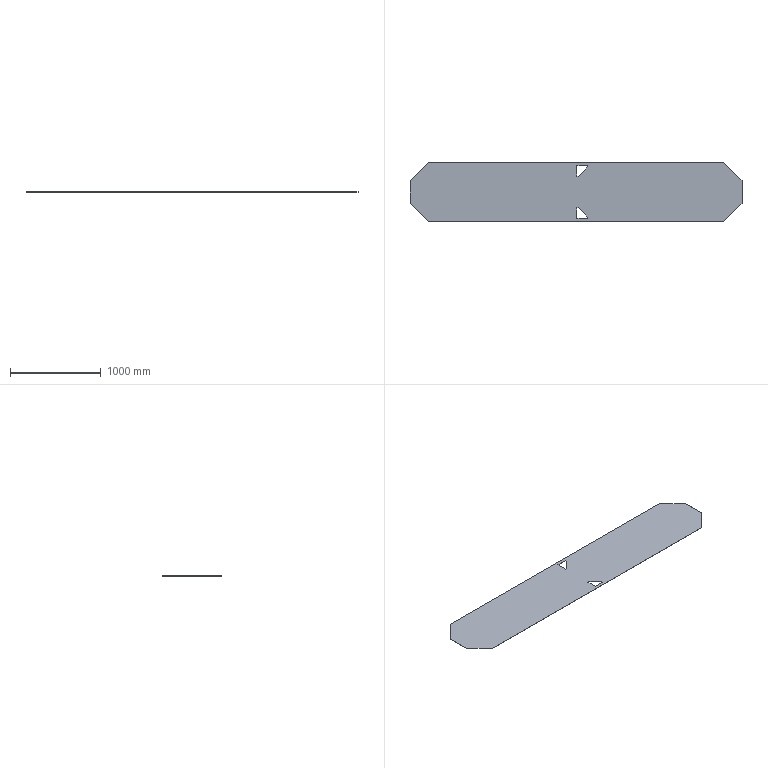Part | STEP file | Bottom weld seal plate2 | 1 solid | 20 faces | box 3650 x 650 x 2 mm | volume 4552100 mm3 | plane 20
STEP:
#1=CARTESIAN_POINT('',(0.,0.,0.));
#2=DIRECTION('',(0.,0.,1.));
#3=DIRECTION('',(1.,0.,0.));
#4=AXIS2_PLACEMENT_3D('',#1,#2,#3);
#5=CARTESIAN_POINT('',(-25.,125.,2.));
#6=VERTEX_POINT('',#5);
#7=CARTESIAN_POINT('',(-25.,-125.,2.));
#8=VERTEX_POINT('',#7);
#9=CARTESIAN_POINT('',(-25.,-125.,2.));
#10=DIRECTION('',(0.,-1.,0.));
#11=VECTOR('',#10,1.);
#12=LINE('',#9,#11);
#13=CARTESIAN_POINT('',(0.,0.,2.));
#14=DIRECTION('',(0.,0.,1.));
#15=DIRECTION('',(1.,0.,0.));
#16=AXIS2_PLACEMENT_3D('',#13,#14,#15);
#17=PLANE('',#16);
#18=CARTESIAN_POINT('',(-25.,-125.));
#19=DIRECTION('',(0.,-1.));
#20=VECTOR('',#19,1.);
#21=LINE('',#18,#20);
#22=(GEOMETRIC_REPRESENTATION_CONTEXT(2)PARAMETRIC_REPRESENTATION_CONTEXT()REPRESENTATION_CONTEXT('',''));
#23=DEFINITIONAL_REPRESENTATION('',(#21),#22);
#24=PCURVE('',#17,#23);
#25=CARTESIAN_POINT('',(-25.,-125.,2.));
#26=DIRECTION('',(1.,0.,0.));
#27=DIRECTION('',(0.,1.,0.));
#28=AXIS2_PLACEMENT_3D('',#25,#26,#27);
#29=PLANE('',#28);
#30=CARTESIAN_POINT('',(0.,0.));
#31=DIRECTION('',(-1.,0.));
#32=VECTOR('',#31,1.);
#33=LINE('',#30,#32);
#34=(GEOMETRIC_REPRESENTATION_CONTEXT(2)PARAMETRIC_REPRESENTATION_CONTEXT()REPRESENTATION_CONTEXT('',''));
#35=DEFINITIONAL_REPRESENTATION('',(#33),#34);
#36=PCURVE('',#29,#35);
#37=SURFACE_CURVE('',#12,(#24,#36),.PCURVE_S1.);
#38=EDGE_CURVE('',#6,#8,#37,.T.);
#39=ORIENTED_EDGE('',*,*,#38,.T.);
#40=CARTESIAN_POINT('',(175.,-325.,2.));
#41=VERTEX_POINT('',#40);
#42=CARTESIAN_POINT('',(-25.,-125.,2.));
#43=DIRECTION('',(0.7071,-0.7071,0.));
#44=VECTOR('',#43,1.);
#45=LINE('',#42,#44);
#46=CARTESIAN_POINT('',(-25.,-125.));
#47=DIRECTION('',(0.7071,-0.7071));
#48=VECTOR('',#47,1.);
#49=LINE('',#46,#48);
#50=(GEOMETRIC_REPRESENTATION_CONTEXT(2)PARAMETRIC_REPRESENTATION_CONTEXT()REPRESENTATION_CONTEXT('',''));
#51=DEFINITIONAL_REPRESENTATION('',(#49),#50);
#52=PCURVE('',#17,#51);
#53=CARTESIAN_POINT('',(-25.,-125.,2.));
#54=DIRECTION('',(0.7071,0.7071,0.));
#55=DIRECTION('',(-0.7071,0.7071,0.));
#56=AXIS2_PLACEMENT_3D('',#53,#54,#55);
#57=PLANE('',#56);
#58=CARTESIAN_POINT('',(0.,0.));
#59=DIRECTION('',(-1.,0.));
#60=VECTOR('',#59,1.);
#61=LINE('',#58,#60);
#62=(GEOMETRIC_REPRESENTATION_CONTEXT(2)PARAMETRIC_REPRESENTATION_CONTEXT()REPRESENTATION_CONTEXT('',''));
#63=DEFINITIONAL_REPRESENTATION('',(#61),#62);
#64=PCURVE('',#57,#63);
#65=SURFACE_CURVE('',#45,(#52,#64),.PCURVE_S1.);
#66=EDGE_CURVE('',#8,#41,#65,.T.);
#67=ORIENTED_EDGE('',*,*,#66,.T.);
#68=CARTESIAN_POINT('',(3425.,-325.,2.));
#69=VERTEX_POINT('',#68);
#70=CARTESIAN_POINT('',(175.,-325.,2.));
#71=DIRECTION('',(1.,0.,0.));
#72=VECTOR('',#71,1.);
#73=LINE('',#70,#72);
#74=CARTESIAN_POINT('',(175.,-325.));
#75=DIRECTION('',(1.,0.));
#76=VECTOR('',#75,1.);
#77=LINE('',#74,#76);
#78=(GEOMETRIC_REPRESENTATION_CONTEXT(2)PARAMETRIC_REPRESENTATION_CONTEXT()REPRESENTATION_CONTEXT('',''));
#79=DEFINITIONAL_REPRESENTATION('',(#77),#78);
#80=PCURVE('',#17,#79);
#81=CARTESIAN_POINT('',(175.,-325.,2.));
#82=DIRECTION('',(0.,1.,0.));
#83=DIRECTION('',(0.,0.,1.));
#84=AXIS2_PLACEMENT_3D('',#81,#82,#83);
#85=PLANE('',#84);
#86=CARTESIAN_POINT('',(0.,0.));
#87=DIRECTION('',(0.,1.));
#88=VECTOR('',#87,1.);
#89=LINE('',#86,#88);
#90=(GEOMETRIC_REPRESENTATION_CONTEXT(2)PARAMETRIC_REPRESENTATION_CONTEXT()REPRESENTATION_CONTEXT('',''));
#91=DEFINITIONAL_REPRESENTATION('',(#89),#90);
#92=PCURVE('',#85,#91);
#93=SURFACE_CURVE('',#73,(#80,#92),.PCURVE_S1.);
#94=EDGE_CURVE('',#41,#69,#93,.T.);
#95=ORIENTED_EDGE('',*,*,#94,.T.);
#96=CARTESIAN_POINT('',(3625.,-125.,2.));
#97=VERTEX_POINT('',#96);
#98=CARTESIAN_POINT('',(3425.,-325.,2.));
#99=DIRECTION('',(0.7071,0.7071,0.));
#100=VECTOR('',#99,1.);
#101=LINE('',#98,#100);
#102=CARTESIAN_POINT('',(3425.,-325.));
#103=DIRECTION('',(0.7071,0.7071));
#104=VECTOR('',#103,1.);
#105=LINE('',#102,#104);
#106=(GEOMETRIC_REPRESENTATION_CONTEXT(2)PARAMETRIC_REPRESENTATION_CONTEXT()REPRESENTATION_CONTEXT('',''));
#107=DEFINITIONAL_REPRESENTATION('',(#105),#106);
#108=PCURVE('',#17,#107);
#109=CARTESIAN_POINT('',(3425.,-325.,2.));
#110=DIRECTION('',(-0.7071,0.7071,0.));
#111=DIRECTION('',(-0.7071,-0.7071,0.));
#112=AXIS2_PLACEMENT_3D('',#109,#110,#111);
#113=PLANE('',#112);
#114=CARTESIAN_POINT('',(0.,0.));
#115=DIRECTION('',(-1.,0.));
#116=VECTOR('',#115,1.);
#117=LINE('',#114,#116);
#118=(GEOMETRIC_REPRESENTATION_CONTEXT(2)PARAMETRIC_REPRESENTATION_CONTEXT()REPRESENTATION_CONTEXT('',''));
#119=DEFINITIONAL_REPRESENTATION('',(#117),#118);
#120=PCURVE('',#113,#119);
#121=SURFACE_CURVE('',#101,(#108,#120),.PCURVE_S1.);
#122=EDGE_CURVE('',#69,#97,#121,.T.);
#123=ORIENTED_EDGE('',*,*,#122,.T.);
#124=CARTESIAN_POINT('',(3625.,125.,2.));
#125=VERTEX_POINT('',#124);
#126=CARTESIAN_POINT('',(3625.,-125.,2.));
#127=DIRECTION('',(0.,1.,0.));
#128=VECTOR('',#127,1.);
#129=LINE('',#126,#128);
#130=CARTESIAN_POINT('',(3625.,-125.));
#131=DIRECTION('',(0.,1.));
#132=VECTOR('',#131,1.);
#133=LINE('',#130,#132);
#134=(GEOMETRIC_REPRESENTATION_CONTEXT(2)PARAMETRIC_REPRESENTATION_CONTEXT()REPRESENTATION_CONTEXT('',''));
#135=DEFINITIONAL_REPRESENTATION('',(#133),#134);
#136=PCURVE('',#17,#135);
#137=CARTESIAN_POINT('',(3625.,-125.,2.));
#138=DIRECTION('',(-1.,0.,0.));
#139=DIRECTION('',(0.,-1.,0.));
#140=AXIS2_PLACEMENT_3D('',#137,#138,#139);
#141=PLANE('',#140);
#142=CARTESIAN_POINT('',(0.,0.));
#143=DIRECTION('',(-1.,0.));
#144=VECTOR('',#143,1.);
#145=LINE('',#142,#144);
#146=(GEOMETRIC_REPRESENTATION_CONTEXT(2)PARAMETRIC_REPRESENTATION_CONTEXT()REPRESENTATION_CONTEXT('',''));
#147=DEFINITIONAL_REPRESENTATION('',(#145),#146);
#148=PCURVE('',#141,#147);
#149=SURFACE_CURVE('',#129,(#136,#148),.PCURVE_S1.);
#150=EDGE_CURVE('',#97,#125,#149,.T.);
#151=ORIENTED_EDGE('',*,*,#150,.T.);
#152=CARTESIAN_POINT('',(3425.,325.,2.));
#153=VERTEX_POINT('',#152);
#154=CARTESIAN_POINT('',(3625.,125.,2.));
#155=DIRECTION('',(-0.7071,0.7071,0.));
#156=VECTOR('',#155,1.);
#157=LINE('',#154,#156);
#158=CARTESIAN_POINT('',(3625.,125.));
#159=DIRECTION('',(-0.7071,0.7071));
#160=VECTOR('',#159,1.);
#161=LINE('',#158,#160);
#162=(GEOMETRIC_REPRESENTATION_CONTEXT(2)PARAMETRIC_REPRESENTATION_CONTEXT()REPRESENTATION_CONTEXT('',''));
#163=DEFINITIONAL_REPRESENTATION('',(#161),#162);
#164=PCURVE('',#17,#163);
#165=CARTESIAN_POINT('',(3625.,125.,2.));
#166=DIRECTION('',(-0.7071,-0.7071,0.));
#167=DIRECTION('',(0.7071,-0.7071,0.));
#168=AXIS2_PLACEMENT_3D('',#165,#166,#167);
#169=PLANE('',#168);
#170=CARTESIAN_POINT('',(0.,0.));
#171=DIRECTION('',(-1.,0.));
#172=VECTOR('',#171,1.);
#173=LINE('',#170,#172);
#174=(GEOMETRIC_REPRESENTATION_CONTEXT(2)PARAMETRIC_REPRESENTATION_CONTEXT()REPRESENTATION_CONTEXT('',''));
#175=DEFINITIONAL_REPRESENTATION('',(#173),#174);
#176=PCURVE('',#169,#175);
#177=SURFACE_CURVE('',#157,(#164,#176),.PCURVE_S1.);
#178=EDGE_CURVE('',#125,#153,#177,.T.);
#179=ORIENTED_EDGE('',*,*,#178,.T.);
#180=CARTESIAN_POINT('',(175.,325.,2.));
#181=VERTEX_POINT('',#180);
#182=CARTESIAN_POINT('',(3425.,325.,2.));
#183=DIRECTION('',(-1.,0.,0.));
#184=VECTOR('',#183,1.);
#185=LINE('',#182,#184);
#186=CARTESIAN_POINT('',(3425.,325.));
#187=DIRECTION('',(-1.,0.));
#188=VECTOR('',#187,1.);
#189=LINE('',#186,#188);
#190=(GEOMETRIC_REPRESENTATION_CONTEXT(2)PARAMETRIC_REPRESENTATION_CONTEXT()REPRESENTATION_CONTEXT('',''));
#191=DEFINITIONAL_REPRESENTATION('',(#189),#190);
#192=PCURVE('',#17,#191);
#193=CARTESIAN_POINT('',(3425.,325.,2.));
#194=DIRECTION('',(0.,-1.,0.));
#195=DIRECTION('',(1.,0.,0.));
#196=AXIS2_PLACEMENT_3D('',#193,#194,#195);
#197=PLANE('',#196);
#198=CARTESIAN_POINT('',(0.,0.));
#199=DIRECTION('',(-1.,0.));
#200=VECTOR('',#199,1.);
#201=LINE('',#198,#200);
#202=(GEOMETRIC_REPRESENTATION_CONTEXT(2)PARAMETRIC_REPRESENTATION_CONTEXT()REPRESENTATION_CONTEXT('',''));
#203=DEFINITIONAL_REPRESENTATION('',(#201),#202);
#204=PCURVE('',#197,#203);
#205=SURFACE_CURVE('',#185,(#192,#204),.PCURVE_S1.);
#206=EDGE_CURVE('',#153,#181,#205,.T.);
#207=ORIENTED_EDGE('',*,*,#206,.T.);
#208=CARTESIAN_POINT('',(175.,325.,2.));
#209=DIRECTION('',(-0.7071,-0.7071,0.));
#210=VECTOR('',#209,1.);
#211=LINE('',#208,#210);
#212=CARTESIAN_POINT('',(175.,325.));
#213=DIRECTION('',(-0.7071,-0.7071));
#214=VECTOR('',#213,1.);
#215=LINE('',#212,#214);
#216=(GEOMETRIC_REPRESENTATION_CONTEXT(2)PARAMETRIC_REPRESENTATION_CONTEXT()REPRESENTATION_CONTEXT('',''));
#217=DEFINITIONAL_REPRESENTATION('',(#215),#216);
#218=PCURVE('',#17,#217);
#219=CARTESIAN_POINT('',(175.,325.,2.));
#220=DIRECTION('',(0.7071,-0.7071,0.));
#221=DIRECTION('',(0.7071,0.7071,0.));
#222=AXIS2_PLACEMENT_3D('',#219,#220,#221);
#223=PLANE('',#222);
#224=CARTESIAN_POINT('',(0.,0.));
#225=DIRECTION('',(-1.,0.));
#226=VECTOR('',#225,1.);
#227=LINE('',#224,#226);
#228=(GEOMETRIC_REPRESENTATION_CONTEXT(2)PARAMETRIC_REPRESENTATION_CONTEXT()REPRESENTATION_CONTEXT('',''));
#229=DEFINITIONAL_REPRESENTATION('',(#227),#228);
#230=PCURVE('',#223,#229);
#231=SURFACE_CURVE('',#211,(#218,#230),.PCURVE_S1.);
#232=EDGE_CURVE('',#181,#6,#231,.T.);
#233=ORIENTED_EDGE('',*,*,#232,.T.);
#234=EDGE_LOOP('',(#39,#67,#95,#123,#151,#179,#207,#233));
#235=FACE_BOUND('',#234,.T.);
#236=CARTESIAN_POINT('',(1810.,175.,2.));
#237=VERTEX_POINT('',#236);
#238=CARTESIAN_POINT('',(1825.,175.,2.));
#239=VERTEX_POINT('',#238);
#240=CARTESIAN_POINT('',(1825.,175.,2.));
#241=DIRECTION('',(1.,0.,0.));
#242=VECTOR('',#241,1.);
#243=LINE('',#240,#242);
#244=CARTESIAN_POINT('',(1825.,175.));
#245=DIRECTION('',(1.,0.));
#246=VECTOR('',#245,1.);
#247=LINE('',#244,#246);
#248=(GEOMETRIC_REPRESENTATION_CONTEXT(2)PARAMETRIC_REPRESENTATION_CONTEXT()REPRESENTATION_CONTEXT('',''));
#249=DEFINITIONAL_REPRESENTATION('',(#247),#248);
#250=PCURVE('',#17,#249);
#251=CARTESIAN_POINT('',(1825.,175.,2.));
#252=DIRECTION('',(0.,1.,0.));
#253=DIRECTION('',(0.,0.,1.));
#254=AXIS2_PLACEMENT_3D('',#251,#252,#253);
#255=PLANE('',#254);
#256=CARTESIAN_POINT('',(0.,0.));
#257=DIRECTION('',(0.,1.));
#258=VECTOR('',#257,1.);
#259=LINE('',#256,#258);
#260=(GEOMETRIC_REPRESENTATION_CONTEXT(2)PARAMETRIC_REPRESENTATION_CONTEXT()REPRESENTATION_CONTEXT('',''));
#261=DEFINITIONAL_REPRESENTATION('',(#259),#260);
#262=PCURVE('',#255,#261);
#263=SURFACE_CURVE('',#243,(#250,#262),.PCURVE_S1.);
#264=EDGE_CURVE('',#237,#239,#263,.T.);
#265=ORIENTED_EDGE('',*,*,#264,.F.);
#266=CARTESIAN_POINT('',(1810.,290.,2.));
#267=VERTEX_POINT('',#266);
#268=CARTESIAN_POINT('',(1810.,175.,2.));
#269=DIRECTION('',(0.,-1.,0.));
#270=VECTOR('',#269,1.);
#271=LINE('',#268,#270);
#272=CARTESIAN_POINT('',(1810.,175.));
#273=DIRECTION('',(0.,-1.));
#274=VECTOR('',#273,1.);
#275=LINE('',#272,#274);
#276=(GEOMETRIC_REPRESENTATION_CONTEXT(2)PARAMETRIC_REPRESENTATION_CONTEXT()REPRESENTATION_CONTEXT('',''));
#277=DEFINITIONAL_REPRESENTATION('',(#275),#276);
#278=PCURVE('',#17,#277);
#279=CARTESIAN_POINT('',(1810.,175.,2.));
#280=DIRECTION('',(1.,0.,0.));
#281=DIRECTION('',(0.,0.,-1.));
#282=AXIS2_PLACEMENT_3D('',#279,#280,#281);
#283=PLANE('',#282);
#284=CARTESIAN_POINT('',(0.,0.));
#285=DIRECTION('',(0.,-1.));
#286=VECTOR('',#285,1.);
#287=LINE('',#284,#286);
#288=(GEOMETRIC_REPRESENTATION_CONTEXT(2)PARAMETRIC_REPRESENTATION_CONTEXT()REPRESENTATION_CONTEXT('',''));
#289=DEFINITIONAL_REPRESENTATION('',(#287),#288);
#290=PCURVE('',#283,#289);
#291=SURFACE_CURVE('',#271,(#278,#290),.PCURVE_S1.);
#292=EDGE_CURVE('',#267,#237,#291,.T.);
#293=ORIENTED_EDGE('',*,*,#292,.F.);
#294=CARTESIAN_POINT('',(1925.,290.,2.));
#295=VERTEX_POINT('',#294);
#296=CARTESIAN_POINT('',(1810.,290.,2.));
#297=DIRECTION('',(-1.,0.,0.));
#298=VECTOR('',#297,1.);
#299=LINE('',#296,#298);
#300=CARTESIAN_POINT('',(1810.,290.));
#301=DIRECTION('',(-1.,0.));
#302=VECTOR('',#301,1.);
#303=LINE('',#300,#302);
#304=(GEOMETRIC_REPRESENTATION_CONTEXT(2)PARAMETRIC_REPRESENTATION_CONTEXT()REPRESENTATION_CONTEXT('',''));
#305=DEFINITIONAL_REPRESENTATION('',(#303),#304);
#306=PCURVE('',#17,#305);
#307=CARTESIAN_POINT('',(1810.,290.,2.));
#308=DIRECTION('',(0.,-1.,0.));
#309=DIRECTION('',(0.,0.,-1.));
#310=AXIS2_PLACEMENT_3D('',#307,#308,#309);
#311=PLANE('',#310);
#312=CARTESIAN_POINT('',(0.,0.));
#313=DIRECTION('',(0.,-1.));
#314=VECTOR('',#313,1.);
#315=LINE('',#312,#314);
#316=(GEOMETRIC_REPRESENTATION_CONTEXT(2)PARAMETRIC_REPRESENTATION_CONTEXT()REPRESENTATION_CONTEXT('',''));
#317=DEFINITIONAL_REPRESENTATION('',(#315),#316);
#318=PCURVE('',#311,#317);
#319=SURFACE_CURVE('',#299,(#306,#318),.PCURVE_S1.);
#320=EDGE_CURVE('',#295,#267,#319,.T.);
#321=ORIENTED_EDGE('',*,*,#320,.F.);
#322=CARTESIAN_POINT('',(1925.,275.,2.));
#323=VERTEX_POINT('',#322);
#324=CARTESIAN_POINT('',(1925.,290.,2.));
#325=DIRECTION('',(0.,1.,0.));
#326=VECTOR('',#325,1.);
#327=LINE('',#324,#326);
#328=CARTESIAN_POINT('',(1925.,290.));
#329=DIRECTION('',(0.,1.));
#330=VECTOR('',#329,1.);
#331=LINE('',#328,#330);
#332=(GEOMETRIC_REPRESENTATION_CONTEXT(2)PARAMETRIC_REPRESENTATION_CONTEXT()REPRESENTATION_CONTEXT('',''));
#333=DEFINITIONAL_REPRESENTATION('',(#331),#332);
#334=PCURVE('',#17,#333);
#335=CARTESIAN_POINT('',(1925.,290.,2.));
#336=DIRECTION('',(-1.,0.,0.));
#337=DIRECTION('',(0.,0.,1.));
#338=AXIS2_PLACEMENT_3D('',#335,#336,#337);
#339=PLANE('',#338);
#340=CARTESIAN_POINT('',(0.,0.));
#341=DIRECTION('',(0.,1.));
#342=VECTOR('',#341,1.);
#343=LINE('',#340,#342);
#344=(GEOMETRIC_REPRESENTATION_CONTEXT(2)PARAMETRIC_REPRESENTATION_CONTEXT()REPRESENTATION_CONTEXT('',''));
#345=DEFINITIONAL_REPRESENTATION('',(#343),#344);
#346=PCURVE('',#339,#345);
#347=SURFACE_CURVE('',#327,(#334,#346),.PCURVE_S1.);
#348=EDGE_CURVE('',#323,#295,#347,.T.);
#349=ORIENTED_EDGE('',*,*,#348,.F.);
#350=CARTESIAN_POINT('',(1925.,275.,2.));
#351=DIRECTION('',(0.7071,0.7071,0.));
#352=VECTOR('',#351,1.);
#353=LINE('',#350,#352);
#354=CARTESIAN_POINT('',(1925.,275.));
#355=DIRECTION('',(0.7071,0.7071));
#356=VECTOR('',#355,1.);
#357=LINE('',#354,#356);
#358=(GEOMETRIC_REPRESENTATION_CONTEXT(2)PARAMETRIC_REPRESENTATION_CONTEXT()REPRESENTATION_CONTEXT('',''));
#359=DEFINITIONAL_REPRESENTATION('',(#357),#358);
#360=PCURVE('',#17,#359);
#361=CARTESIAN_POINT('',(1925.,275.,2.));
#362=DIRECTION('',(-0.7071,0.7071,0.));
#363=DIRECTION('',(-0.7071,-0.7071,0.));
#364=AXIS2_PLACEMENT_3D('',#361,#362,#363);
#365=PLANE('',#364);
#366=CARTESIAN_POINT('',(0.,0.));
#367=DIRECTION('',(-1.,0.));
#368=VECTOR('',#367,1.);
#369=LINE('',#366,#368);
#370=(GEOMETRIC_REPRESENTATION_CONTEXT(2)PARAMETRIC_REPRESENTATION_CONTEXT()REPRESENTATION_CONTEXT('',''));
#371=DEFINITIONAL_REPRESENTATION('',(#369),#370);
#372=PCURVE('',#365,#371);
#373=SURFACE_CURVE('',#353,(#360,#372),.PCURVE_S1.);
#374=EDGE_CURVE('',#239,#323,#373,.T.);
#375=ORIENTED_EDGE('',*,*,#374,.F.);
#376=EDGE_LOOP('',(#265,#293,#321,#349,#375));
#377=FACE_BOUND('',#376,.T.);
#378=CARTESIAN_POINT('',(1925.,-290.,2.));
#379=VERTEX_POINT('',#378);
#380=CARTESIAN_POINT('',(1925.,-275.,2.));
#381=VERTEX_POINT('',#380);
#382=CARTESIAN_POINT('',(1925.,-290.,2.));
#383=DIRECTION('',(0.,1.,0.));
#384=VECTOR('',#383,1.);
#385=LINE('',#382,#384);
#386=CARTESIAN_POINT('',(1925.,-290.));
#387=DIRECTION('',(0.,1.));
#388=VECTOR('',#387,1.);
#389=LINE('',#386,#388);
#390=(GEOMETRIC_REPRESENTATION_CONTEXT(2)PARAMETRIC_REPRESENTATION_CONTEXT()REPRESENTATION_CONTEXT('',''));
#391=DEFINITIONAL_REPRESENTATION('',(#389),#390);
#392=PCURVE('',#17,#391);
#393=CARTESIAN_POINT('',(1925.,-290.,2.));
#394=DIRECTION('',(-1.,0.,0.));
#395=DIRECTION('',(0.,0.,1.));
#396=AXIS2_PLACEMENT_3D('',#393,#394,#395);
#397=PLANE('',#396);
#398=CARTESIAN_POINT('',(0.,0.));
#399=DIRECTION('',(0.,1.));
#400=VECTOR('',#399,1.);
#401=LINE('',#398,#400);
#402=(GEOMETRIC_REPRESENTATION_CONTEXT(2)PARAMETRIC_REPRESENTATION_CONTEXT()REPRESENTATION_CONTEXT('',''));
#403=DEFINITIONAL_REPRESENTATION('',(#401),#402);
#404=PCURVE('',#397,#403);
#405=SURFACE_CURVE('',#385,(#392,#404),.PCURVE_S1.);
#406=EDGE_CURVE('',#379,#381,#405,.T.);
#407=ORIENTED_EDGE('',*,*,#406,.F.);
#408=CARTESIAN_POINT('',(1810.,-290.,2.));
#409=VERTEX_POINT('',#408);
#410=CARTESIAN_POINT('',(1810.,-290.,2.));
#411=DIRECTION('',(1.,0.,0.));
#412=VECTOR('',#411,1.);
#413=LINE('',#410,#412);
#414=CARTESIAN_POINT('',(1810.,-290.));
#415=DIRECTION('',(1.,0.));
#416=VECTOR('',#415,1.);
#417=LINE('',#414,#416);
#418=(GEOMETRIC_REPRESENTATION_CONTEXT(2)PARAMETRIC_REPRESENTATION_CONTEXT()REPRESENTATION_CONTEXT('',''));
#419=DEFINITIONAL_REPRESENTATION('',(#417),#418);
#420=PCURVE('',#17,#419);
#421=CARTESIAN_POINT('',(1810.,-290.,2.));
#422=DIRECTION('',(0.,1.,0.));
#423=DIRECTION('',(0.,0.,1.));
#424=AXIS2_PLACEMENT_3D('',#421,#422,#423);
#425=PLANE('',#424);
#426=CARTESIAN_POINT('',(0.,0.));
#427=DIRECTION('',(0.,1.));
#428=VECTOR('',#427,1.);
#429=LINE('',#426,#428);
#430=(GEOMETRIC_REPRESENTATION_CONTEXT(2)PARAMETRIC_REPRESENTATION_CONTEXT()REPRESENTATION_CONTEXT('',''));
#431=DEFINITIONAL_REPRESENTATION('',(#429),#430);
#432=PCURVE('',#425,#431);
#433=SURFACE_CURVE('',#413,(#420,#432),.PCURVE_S1.);
#434=EDGE_CURVE('',#409,#379,#433,.T.);
#435=ORIENTED_EDGE('',*,*,#434,.F.);
#436=CARTESIAN_POINT('',(1810.,-175.,2.));
#437=VERTEX_POINT('',#436);
#438=CARTESIAN_POINT('',(1810.,-290.,2.));
#439=DIRECTION('',(0.,-1.,0.));
#440=VECTOR('',#439,1.);
#441=LINE('',#438,#440);
#442=CARTESIAN_POINT('',(1810.,-290.));
#443=DIRECTION('',(0.,-1.));
#444=VECTOR('',#443,1.);
#445=LINE('',#442,#444);
#446=(GEOMETRIC_REPRESENTATION_CONTEXT(2)PARAMETRIC_REPRESENTATION_CONTEXT()REPRESENTATION_CONTEXT('',''));
#447=DEFINITIONAL_REPRESENTATION('',(#445),#446);
#448=PCURVE('',#17,#447);
#449=CARTESIAN_POINT('',(1810.,-290.,2.));
#450=DIRECTION('',(1.,0.,0.));
#451=DIRECTION('',(0.,0.,-1.));
#452=AXIS2_PLACEMENT_3D('',#449,#450,#451);
#453=PLANE('',#452);
#454=CARTESIAN_POINT('',(0.,0.));
#455=DIRECTION('',(0.,-1.));
#456=VECTOR('',#455,1.);
#457=LINE('',#454,#456);
#458=(GEOMETRIC_REPRESENTATION_CONTEXT(2)PARAMETRIC_REPRESENTATION_CONTEXT()REPRESENTATION_CONTEXT('',''));
#459=DEFINITIONAL_REPRESENTATION('',(#457),#458);
#460=PCURVE('',#453,#459);
#461=SURFACE_CURVE('',#441,(#448,#460),.PCURVE_S1.);
#462=EDGE_CURVE('',#437,#409,#461,.T.);
#463=ORIENTED_EDGE('',*,*,#462,.F.);
#464=CARTESIAN_POINT('',(1825.,-175.,2.));
#465=VERTEX_POINT('',#464);
#466=CARTESIAN_POINT('',(1825.,-175.,2.));
#467=DIRECTION('',(-1.,0.,0.));
#468=VECTOR('',#467,1.);
#469=LINE('',#466,#468);
#470=CARTESIAN_POINT('',(1825.,-175.));
#471=DIRECTION('',(-1.,0.));
#472=VECTOR('',#471,1.);
#473=LINE('',#470,#472);
#474=(GEOMETRIC_REPRESENTATION_CONTEXT(2)PARAMETRIC_REPRESENTATION_CONTEXT()REPRESENTATION_CONTEXT('',''));
#475=DEFINITIONAL_REPRESENTATION('',(#473),#474);
#476=PCURVE('',#17,#475);
#477=CARTESIAN_POINT('',(1825.,-175.,2.));
#478=DIRECTION('',(0.,-1.,0.));
#479=DIRECTION('',(0.,0.,-1.));
#480=AXIS2_PLACEMENT_3D('',#477,#478,#479);
#481=PLANE('',#480);
#482=CARTESIAN_POINT('',(0.,0.));
#483=DIRECTION('',(0.,-1.));
#484=VECTOR('',#483,1.);
#485=LINE('',#482,#484);
#486=(GEOMETRIC_REPRESENTATION_CONTEXT(2)PARAMETRIC_REPRESENTATION_CONTEXT()REPRESENTATION_CONTEXT('',''));
#487=DEFINITIONAL_REPRESENTATION('',(#485),#486);
#488=PCURVE('',#481,#487);
#489=SURFACE_CURVE('',#469,(#476,#488),.PCURVE_S1.);
#490=EDGE_CURVE('',#465,#437,#489,.T.);
#491=ORIENTED_EDGE('',*,*,#490,.F.);
#492=CARTESIAN_POINT('',(1925.,-275.,2.));
#493=DIRECTION('',(-0.7071,0.7071,0.));
#494=VECTOR('',#493,1.);
#495=LINE('',#492,#494);
#496=CARTESIAN_POINT('',(1925.,-275.));
#497=DIRECTION('',(-0.7071,0.7071));
#498=VECTOR('',#497,1.);
#499=LINE('',#496,#498);
#500=(GEOMETRIC_REPRESENTATION_CONTEXT(2)PARAMETRIC_REPRESENTATION_CONTEXT()REPRESENTATION_CONTEXT('',''));
#501=DEFINITIONAL_REPRESENTATION('',(#499),#500);
#502=PCURVE('',#17,#501);
#503=CARTESIAN_POINT('',(1925.,-275.,2.));
#504=DIRECTION('',(-0.7071,-0.7071,0.));
#505=DIRECTION('',(0.7071,-0.7071,0.));
#506=AXIS2_PLACEMENT_3D('',#503,#504,#505);
#507=PLANE('',#506);
#508=CARTESIAN_POINT('',(0.,0.));
#509=DIRECTION('',(-1.,0.));
#510=VECTOR('',#509,1.);
#511=LINE('',#508,#510);
#512=(GEOMETRIC_REPRESENTATION_CONTEXT(2)PARAMETRIC_REPRESENTATION_CONTEXT()REPRESENTATION_CONTEXT('',''));
#513=DEFINITIONAL_REPRESENTATION('',(#511),#512);
#514=PCURVE('',#507,#513);
#515=SURFACE_CURVE('',#495,(#502,#514),.PCURVE_S1.);
#516=EDGE_CURVE('',#381,#465,#515,.T.);
#517=ORIENTED_EDGE('',*,*,#516,.F.);
#518=EDGE_LOOP('',(#407,#435,#463,#491,#517));
#519=FACE_BOUND('',#518,.T.);
#520=ADVANCED_FACE('',(#235,#377,#519),#17,.T.);
#521=CARTESIAN_POINT('',(1810.,290.,0.));
#522=VERTEX_POINT('',#521);
#523=CARTESIAN_POINT('',(1810.,175.,0.));
#524=VERTEX_POINT('',#523);
#525=CARTESIAN_POINT('',(1810.,175.,0.));
#526=DIRECTION('',(0.,-1.,0.));
#527=VECTOR('',#526,1.);
#528=LINE('',#525,#527);
#529=CARTESIAN_POINT('',(0.,0.,0.));
#530=DIRECTION('',(0.,0.,1.));
#531=DIRECTION('',(1.,0.,0.));
#532=AXIS2_PLACEMENT_3D('',#529,#530,#531);
#533=PLANE('',#532);
#534=CARTESIAN_POINT('',(1810.,175.));
#535=DIRECTION('',(0.,-1.));
#536=VECTOR('',#535,1.);
#537=LINE('',#534,#536);
#538=(GEOMETRIC_REPRESENTATION_CONTEXT(2)PARAMETRIC_REPRESENTATION_CONTEXT()REPRESENTATION_CONTEXT('',''));
#539=DEFINITIONAL_REPRESENTATION('',(#537),#538);
#540=PCURVE('',#533,#539);
#541=CARTESIAN_POINT('',(2.,0.));
#542=DIRECTION('',(0.,-1.));
#543=VECTOR('',#542,1.);
#544=LINE('',#541,#543);
#545=(GEOMETRIC_REPRESENTATION_CONTEXT(2)PARAMETRIC_REPRESENTATION_CONTEXT()REPRESENTATION_CONTEXT('',''));
#546=DEFINITIONAL_REPRESENTATION('',(#544),#545);
#547=PCURVE('',#283,#546);
#548=SURFACE_CURVE('',#528,(#540,#547),.PCURVE_S1.);
#549=EDGE_CURVE('',#522,#524,#548,.T.);
#550=ORIENTED_EDGE('',*,*,#549,.T.);
#551=CARTESIAN_POINT('',(1825.,175.,0.));
#552=VERTEX_POINT('',#551);
#553=CARTESIAN_POINT('',(1825.,175.,0.));
#554=DIRECTION('',(1.,0.,0.));
#555=VECTOR('',#554,1.);
#556=LINE('',#553,#555);
#557=CARTESIAN_POINT('',(1825.,175.));
#558=DIRECTION('',(1.,0.));
#559=VECTOR('',#558,1.);
#560=LINE('',#557,#559);
#561=(GEOMETRIC_REPRESENTATION_CONTEXT(2)PARAMETRIC_REPRESENTATION_CONTEXT()REPRESENTATION_CONTEXT('',''));
#562=DEFINITIONAL_REPRESENTATION('',(#560),#561);
#563=PCURVE('',#533,#562);
#564=CARTESIAN_POINT('',(-2.,0.));
#565=DIRECTION('',(0.,1.));
#566=VECTOR('',#565,1.);
#567=LINE('',#564,#566);
#568=(GEOMETRIC_REPRESENTATION_CONTEXT(2)PARAMETRIC_REPRESENTATION_CONTEXT()REPRESENTATION_CONTEXT('',''));
#569=DEFINITIONAL_REPRESENTATION('',(#567),#568);
#570=PCURVE('',#255,#569);
#571=SURFACE_CURVE('',#556,(#563,#570),.PCURVE_S1.);
#572=EDGE_CURVE('',#524,#552,#571,.T.);
#573=ORIENTED_EDGE('',*,*,#572,.T.);
#574=CARTESIAN_POINT('',(1925.,275.,0.));
#575=VERTEX_POINT('',#574);
#576=CARTESIAN_POINT('',(1925.,275.,0.));
#577=DIRECTION('',(0.7071,0.7071,0.));
#578=VECTOR('',#577,1.);
#579=LINE('',#576,#578);
#580=CARTESIAN_POINT('',(1925.,275.));
#581=DIRECTION('',(0.7071,0.7071));
#582=VECTOR('',#581,1.);
#583=LINE('',#580,#582);
#584=(GEOMETRIC_REPRESENTATION_CONTEXT(2)PARAMETRIC_REPRESENTATION_CONTEXT()REPRESENTATION_CONTEXT('',''));
#585=DEFINITIONAL_REPRESENTATION('',(#583),#584);
#586=PCURVE('',#533,#585);
#587=CARTESIAN_POINT('',(0.,-2.));
#588=DIRECTION('',(-1.,0.));
#589=VECTOR('',#588,1.);
#590=LINE('',#587,#589);
#591=(GEOMETRIC_REPRESENTATION_CONTEXT(2)PARAMETRIC_REPRESENTATION_CONTEXT()REPRESENTATION_CONTEXT('',''));
#592=DEFINITIONAL_REPRESENTATION('',(#590),#591);
#593=PCURVE('',#365,#592);
#594=SURFACE_CURVE('',#579,(#586,#593),.PCURVE_S1.);
#595=EDGE_CURVE('',#552,#575,#594,.T.);
#596=ORIENTED_EDGE('',*,*,#595,.T.);
#597=CARTESIAN_POINT('',(1925.,290.,0.));
#598=VERTEX_POINT('',#597);
#599=CARTESIAN_POINT('',(1925.,290.,0.));
#600=DIRECTION('',(0.,1.,0.));
#601=VECTOR('',#600,1.);
#602=LINE('',#599,#601);
#603=CARTESIAN_POINT('',(1925.,290.));
#604=DIRECTION('',(0.,1.));
#605=VECTOR('',#604,1.);
#606=LINE('',#603,#605);
#607=(GEOMETRIC_REPRESENTATION_CONTEXT(2)PARAMETRIC_REPRESENTATION_CONTEXT()REPRESENTATION_CONTEXT('',''));
#608=DEFINITIONAL_REPRESENTATION('',(#606),#607);
#609=PCURVE('',#533,#608);
#610=CARTESIAN_POINT('',(-2.,0.));
#611=DIRECTION('',(0.,1.));
#612=VECTOR('',#611,1.);
#613=LINE('',#610,#612);
#614=(GEOMETRIC_REPRESENTATION_CONTEXT(2)PARAMETRIC_REPRESENTATION_CONTEXT()REPRESENTATION_CONTEXT('',''));
#615=DEFINITIONAL_REPRESENTATION('',(#613),#614);
#616=PCURVE('',#339,#615);
#617=SURFACE_CURVE('',#602,(#609,#616),.PCURVE_S1.);
#618=EDGE_CURVE('',#575,#598,#617,.T.);
#619=ORIENTED_EDGE('',*,*,#618,.T.);
#620=CARTESIAN_POINT('',(1810.,290.,0.));
#621=DIRECTION('',(-1.,0.,0.));
#622=VECTOR('',#621,1.);
#623=LINE('',#620,#622);
#624=CARTESIAN_POINT('',(1810.,290.));
#625=DIRECTION('',(-1.,0.));
#626=VECTOR('',#625,1.);
#627=LINE('',#624,#626);
#628=(GEOMETRIC_REPRESENTATION_CONTEXT(2)PARAMETRIC_REPRESENTATION_CONTEXT()REPRESENTATION_CONTEXT('',''));
#629=DEFINITIONAL_REPRESENTATION('',(#627),#628);
#630=PCURVE('',#533,#629);
#631=CARTESIAN_POINT('',(2.,0.));
#632=DIRECTION('',(0.,-1.));
#633=VECTOR('',#632,1.);
#634=LINE('',#631,#633);
#635=(GEOMETRIC_REPRESENTATION_CONTEXT(2)PARAMETRIC_REPRESENTATION_CONTEXT()REPRESENTATION_CONTEXT('',''));
#636=DEFINITIONAL_REPRESENTATION('',(#634),#635);
#637=PCURVE('',#311,#636);
#638=SURFACE_CURVE('',#623,(#630,#637),.PCURVE_S1.);
#639=EDGE_CURVE('',#598,#522,#638,.T.);
#640=ORIENTED_EDGE('',*,*,#639,.T.);
#641=EDGE_LOOP('',(#550,#573,#596,#619,#640));
#642=FACE_BOUND('',#641,.T.);
#643=CARTESIAN_POINT('',(-25.,125.,0.));
#644=VERTEX_POINT('',#643);
#645=CARTESIAN_POINT('',(-25.,-125.,0.));
#646=VERTEX_POINT('',#645);
#647=CARTESIAN_POINT('',(-25.,-125.,0.));
#648=DIRECTION('',(0.,-1.,0.));
#649=VECTOR('',#648,1.);
#650=LINE('',#647,#649);
#651=CARTESIAN_POINT('',(-25.,-125.));
#652=DIRECTION('',(0.,-1.));
#653=VECTOR('',#652,1.);
#654=LINE('',#651,#653);
#655=(GEOMETRIC_REPRESENTATION_CONTEXT(2)PARAMETRIC_REPRESENTATION_CONTEXT()REPRESENTATION_CONTEXT('',''));
#656=DEFINITIONAL_REPRESENTATION('',(#654),#655);
#657=PCURVE('',#533,#656);
#658=CARTESIAN_POINT('',(0.,-2.));
#659=DIRECTION('',(-1.,0.));
#660=VECTOR('',#659,1.);
#661=LINE('',#658,#660);
#662=(GEOMETRIC_REPRESENTATION_CONTEXT(2)PARAMETRIC_REPRESENTATION_CONTEXT()REPRESENTATION_CONTEXT('',''));
#663=DEFINITIONAL_REPRESENTATION('',(#661),#662);
#664=PCURVE('',#29,#663);
#665=SURFACE_CURVE('',#650,(#657,#664),.PCURVE_S1.);
#666=EDGE_CURVE('',#644,#646,#665,.T.);
#667=ORIENTED_EDGE('',*,*,#666,.F.);
#668=CARTESIAN_POINT('',(175.,325.,0.));
#669=VERTEX_POINT('',#668);
#670=CARTESIAN_POINT('',(175.,325.,0.));
#671=DIRECTION('',(-0.7071,-0.7071,0.));
#672=VECTOR('',#671,1.);
#673=LINE('',#670,#672);
#674=CARTESIAN_POINT('',(175.,325.));
#675=DIRECTION('',(-0.7071,-0.7071));
#676=VECTOR('',#675,1.);
#677=LINE('',#674,#676);
#678=(GEOMETRIC_REPRESENTATION_CONTEXT(2)PARAMETRIC_REPRESENTATION_CONTEXT()REPRESENTATION_CONTEXT('',''));
#679=DEFINITIONAL_REPRESENTATION('',(#677),#678);
#680=PCURVE('',#533,#679);
#681=CARTESIAN_POINT('',(0.,-2.));
#682=DIRECTION('',(-1.,0.));
#683=VECTOR('',#682,1.);
#684=LINE('',#681,#683);
#685=(GEOMETRIC_REPRESENTATION_CONTEXT(2)PARAMETRIC_REPRESENTATION_CONTEXT()REPRESENTATION_CONTEXT('',''));
#686=DEFINITIONAL_REPRESENTATION('',(#684),#685);
#687=PCURVE('',#223,#686);
#688=SURFACE_CURVE('',#673,(#680,#687),.PCURVE_S1.);
#689=EDGE_CURVE('',#669,#644,#688,.T.);
#690=ORIENTED_EDGE('',*,*,#689,.F.);
#691=CARTESIAN_POINT('',(3425.,325.,0.));
#692=VERTEX_POINT('',#691);
#693=CARTESIAN_POINT('',(3425.,325.,0.));
#694=DIRECTION('',(-1.,0.,0.));
#695=VECTOR('',#694,1.);
#696=LINE('',#693,#695);
#697=CARTESIAN_POINT('',(3425.,325.));
#698=DIRECTION('',(-1.,0.));
#699=VECTOR('',#698,1.);
#700=LINE('',#697,#699);
#701=(GEOMETRIC_REPRESENTATION_CONTEXT(2)PARAMETRIC_REPRESENTATION_CONTEXT()REPRESENTATION_CONTEXT('',''));
#702=DEFINITIONAL_REPRESENTATION('',(#700),#701);
#703=PCURVE('',#533,#702);
#704=CARTESIAN_POINT('',(0.,-2.));
#705=DIRECTION('',(-1.,0.));
#706=VECTOR('',#705,1.);
#707=LINE('',#704,#706);
#708=(GEOMETRIC_REPRESENTATION_CONTEXT(2)PARAMETRIC_REPRESENTATION_CONTEXT()REPRESENTATION_CONTEXT('',''));
#709=DEFINITIONAL_REPRESENTATION('',(#707),#708);
#710=PCURVE('',#197,#709);
#711=SURFACE_CURVE('',#696,(#703,#710),.PCURVE_S1.);
#712=EDGE_CURVE('',#692,#669,#711,.T.);
#713=ORIENTED_EDGE('',*,*,#712,.F.);
#714=CARTESIAN_POINT('',(3625.,125.,0.));
#715=VERTEX_POINT('',#714);
#716=CARTESIAN_POINT('',(3625.,125.,0.));
#717=DIRECTION('',(-0.7071,0.7071,0.));
#718=VECTOR('',#717,1.);
#719=LINE('',#716,#718);
#720=CARTESIAN_POINT('',(3625.,125.));
#721=DIRECTION('',(-0.7071,0.7071));
#722=VECTOR('',#721,1.);
#723=LINE('',#720,#722);
#724=(GEOMETRIC_REPRESENTATION_CONTEXT(2)PARAMETRIC_REPRESENTATION_CONTEXT()REPRESENTATION_CONTEXT('',''));
#725=DEFINITIONAL_REPRESENTATION('',(#723),#724);
#726=PCURVE('',#533,#725);
#727=CARTESIAN_POINT('',(0.,-2.));
#728=DIRECTION('',(-1.,0.));
#729=VECTOR('',#728,1.);
#730=LINE('',#727,#729);
#731=(GEOMETRIC_REPRESENTATION_CONTEXT(2)PARAMETRIC_REPRESENTATION_CONTEXT()REPRESENTATION_CONTEXT('',''));
#732=DEFINITIONAL_REPRESENTATION('',(#730),#731);
#733=PCURVE('',#169,#732);
#734=SURFACE_CURVE('',#719,(#726,#733),.PCURVE_S1.);
#735=EDGE_CURVE('',#715,#692,#734,.T.);
#736=ORIENTED_EDGE('',*,*,#735,.F.);
#737=CARTESIAN_POINT('',(3625.,-125.,0.));
#738=VERTEX_POINT('',#737);
#739=CARTESIAN_POINT('',(3625.,-125.,0.));
#740=DIRECTION('',(0.,1.,0.));
#741=VECTOR('',#740,1.);
#742=LINE('',#739,#741);
#743=CARTESIAN_POINT('',(3625.,-125.));
#744=DIRECTION('',(0.,1.));
#745=VECTOR('',#744,1.);
#746=LINE('',#743,#745);
#747=(GEOMETRIC_REPRESENTATION_CONTEXT(2)PARAMETRIC_REPRESENTATION_CONTEXT()REPRESENTATION_CONTEXT('',''));
#748=DEFINITIONAL_REPRESENTATION('',(#746),#747);
#749=PCURVE('',#533,#748);
#750=CARTESIAN_POINT('',(0.,-2.));
#751=DIRECTION('',(-1.,0.));
#752=VECTOR('',#751,1.);
#753=LINE('',#750,#752);
#754=(GEOMETRIC_REPRESENTATION_CONTEXT(2)PARAMETRIC_REPRESENTATION_CONTEXT()REPRESENTATION_CONTEXT('',''));
#755=DEFINITIONAL_REPRESENTATION('',(#753),#754);
#756=PCURVE('',#141,#755);
#757=SURFACE_CURVE('',#742,(#749,#756),.PCURVE_S1.);
#758=EDGE_CURVE('',#738,#715,#757,.T.);
#759=ORIENTED_EDGE('',*,*,#758,.F.);
#760=CARTESIAN_POINT('',(3425.,-325.,0.));
#761=VERTEX_POINT('',#760);
#762=CARTESIAN_POINT('',(3425.,-325.,0.));
#763=DIRECTION('',(0.7071,0.7071,0.));
#764=VECTOR('',#763,1.);
#765=LINE('',#762,#764);
#766=CARTESIAN_POINT('',(3425.,-325.));
#767=DIRECTION('',(0.7071,0.7071));
#768=VECTOR('',#767,1.);
#769=LINE('',#766,#768);
#770=(GEOMETRIC_REPRESENTATION_CONTEXT(2)PARAMETRIC_REPRESENTATION_CONTEXT()REPRESENTATION_CONTEXT('',''));
#771=DEFINITIONAL_REPRESENTATION('',(#769),#770);
#772=PCURVE('',#533,#771);
#773=CARTESIAN_POINT('',(0.,-2.));
#774=DIRECTION('',(-1.,0.));
#775=VECTOR('',#774,1.);
#776=LINE('',#773,#775);
#777=(GEOMETRIC_REPRESENTATION_CONTEXT(2)PARAMETRIC_REPRESENTATION_CONTEXT()REPRESENTATION_CONTEXT('',''));
#778=DEFINITIONAL_REPRESENTATION('',(#776),#777);
#779=PCURVE('',#113,#778);
#780=SURFACE_CURVE('',#765,(#772,#779),.PCURVE_S1.);
#781=EDGE_CURVE('',#761,#738,#780,.T.);
#782=ORIENTED_EDGE('',*,*,#781,.F.);
#783=CARTESIAN_POINT('',(175.,-325.,0.));
#784=VERTEX_POINT('',#783);
#785=CARTESIAN_POINT('',(175.,-325.,0.));
#786=DIRECTION('',(1.,0.,0.));
#787=VECTOR('',#786,1.);
#788=LINE('',#785,#787);
#789=CARTESIAN_POINT('',(175.,-325.));
#790=DIRECTION('',(1.,0.));
#791=VECTOR('',#790,1.);
#792=LINE('',#789,#791);
#793=(GEOMETRIC_REPRESENTATION_CONTEXT(2)PARAMETRIC_REPRESENTATION_CONTEXT()REPRESENTATION_CONTEXT('',''));
#794=DEFINITIONAL_REPRESENTATION('',(#792),#793);
#795=PCURVE('',#533,#794);
#796=CARTESIAN_POINT('',(-2.,0.));
#797=DIRECTION('',(0.,1.));
#798=VECTOR('',#797,1.);
#799=LINE('',#796,#798);
#800=(GEOMETRIC_REPRESENTATION_CONTEXT(2)PARAMETRIC_REPRESENTATION_CONTEXT()REPRESENTATION_CONTEXT('',''));
#801=DEFINITIONAL_REPRESENTATION('',(#799),#800);
#802=PCURVE('',#85,#801);
#803=SURFACE_CURVE('',#788,(#795,#802),.PCURVE_S1.);
#804=EDGE_CURVE('',#784,#761,#803,.T.);
#805=ORIENTED_EDGE('',*,*,#804,.F.);
#806=CARTESIAN_POINT('',(-25.,-125.,0.));
#807=DIRECTION('',(0.7071,-0.7071,0.));
#808=VECTOR('',#807,1.);
#809=LINE('',#806,#808);
#810=CARTESIAN_POINT('',(-25.,-125.));
#811=DIRECTION('',(0.7071,-0.7071));
#812=VECTOR('',#811,1.);
#813=LINE('',#810,#812);
#814=(GEOMETRIC_REPRESENTATION_CONTEXT(2)PARAMETRIC_REPRESENTATION_CONTEXT()REPRESENTATION_CONTEXT('',''));
#815=DEFINITIONAL_REPRESENTATION('',(#813),#814);
#816=PCURVE('',#533,#815);
#817=CARTESIAN_POINT('',(0.,-2.));
#818=DIRECTION('',(-1.,0.));
#819=VECTOR('',#818,1.);
#820=LINE('',#817,#819);
#821=(GEOMETRIC_REPRESENTATION_CONTEXT(2)PARAMETRIC_REPRESENTATION_CONTEXT()REPRESENTATION_CONTEXT('',''));
#822=DEFINITIONAL_REPRESENTATION('',(#820),#821);
#823=PCURVE('',#57,#822);
#824=SURFACE_CURVE('',#809,(#816,#823),.PCURVE_S1.);
#825=EDGE_CURVE('',#646,#784,#824,.T.);
#826=ORIENTED_EDGE('',*,*,#825,.F.);
#827=EDGE_LOOP('',(#667,#690,#713,#736,#759,#782,#805,#826));
#828=FACE_BOUND('',#827,.T.);
#829=CARTESIAN_POINT('',(1810.,-290.,0.));
#830=VERTEX_POINT('',#829);
#831=CARTESIAN_POINT('',(1925.,-290.,0.));
#832=VERTEX_POINT('',#831);
#833=CARTESIAN_POINT('',(1810.,-290.,0.));
#834=DIRECTION('',(1.,0.,0.));
#835=VECTOR('',#834,1.);
#836=LINE('',#833,#835);
#837=CARTESIAN_POINT('',(1810.,-290.));
#838=DIRECTION('',(1.,0.));
#839=VECTOR('',#838,1.);
#840=LINE('',#837,#839);
#841=(GEOMETRIC_REPRESENTATION_CONTEXT(2)PARAMETRIC_REPRESENTATION_CONTEXT()REPRESENTATION_CONTEXT('',''));
#842=DEFINITIONAL_REPRESENTATION('',(#840),#841);
#843=PCURVE('',#533,#842);
#844=CARTESIAN_POINT('',(-2.,0.));
#845=DIRECTION('',(0.,1.));
#846=VECTOR('',#845,1.);
#847=LINE('',#844,#846);
#848=(GEOMETRIC_REPRESENTATION_CONTEXT(2)PARAMETRIC_REPRESENTATION_CONTEXT()REPRESENTATION_CONTEXT('',''));
#849=DEFINITIONAL_REPRESENTATION('',(#847),#848);
#850=PCURVE('',#425,#849);
#851=SURFACE_CURVE('',#836,(#843,#850),.PCURVE_S1.);
#852=EDGE_CURVE('',#830,#832,#851,.T.);
#853=ORIENTED_EDGE('',*,*,#852,.T.);
#854=CARTESIAN_POINT('',(1925.,-275.,0.));
#855=VERTEX_POINT('',#854);
#856=CARTESIAN_POINT('',(1925.,-290.,0.));
#857=DIRECTION('',(0.,1.,0.));
#858=VECTOR('',#857,1.);
#859=LINE('',#856,#858);
#860=CARTESIAN_POINT('',(1925.,-290.));
#861=DIRECTION('',(0.,1.));
#862=VECTOR('',#861,1.);
#863=LINE('',#860,#862);
#864=(GEOMETRIC_REPRESENTATION_CONTEXT(2)PARAMETRIC_REPRESENTATION_CONTEXT()REPRESENTATION_CONTEXT('',''));
#865=DEFINITIONAL_REPRESENTATION('',(#863),#864);
#866=PCURVE('',#533,#865);
#867=CARTESIAN_POINT('',(-2.,0.));
#868=DIRECTION('',(0.,1.));
#869=VECTOR('',#868,1.);
#870=LINE('',#867,#869);
#871=(GEOMETRIC_REPRESENTATION_CONTEXT(2)PARAMETRIC_REPRESENTATION_CONTEXT()REPRESENTATION_CONTEXT('',''));
#872=DEFINITIONAL_REPRESENTATION('',(#870),#871);
#873=PCURVE('',#397,#872);
#874=SURFACE_CURVE('',#859,(#866,#873),.PCURVE_S1.);
#875=EDGE_CURVE('',#832,#855,#874,.T.);
#876=ORIENTED_EDGE('',*,*,#875,.T.);
#877=CARTESIAN_POINT('',(1825.,-175.,0.));
#878=VERTEX_POINT('',#877);
#879=CARTESIAN_POINT('',(1925.,-275.,0.));
#880=DIRECTION('',(-0.7071,0.7071,0.));
#881=VECTOR('',#880,1.);
#882=LINE('',#879,#881);
#883=CARTESIAN_POINT('',(1925.,-275.));
#884=DIRECTION('',(-0.7071,0.7071));
#885=VECTOR('',#884,1.);
#886=LINE('',#883,#885);
#887=(GEOMETRIC_REPRESENTATION_CONTEXT(2)PARAMETRIC_REPRESENTATION_CONTEXT()REPRESENTATION_CONTEXT('',''));
#888=DEFINITIONAL_REPRESENTATION('',(#886),#887);
#889=PCURVE('',#533,#888);
#890=CARTESIAN_POINT('',(0.,-2.));
#891=DIRECTION('',(-1.,0.));
#892=VECTOR('',#891,1.);
#893=LINE('',#890,#892);
#894=(GEOMETRIC_REPRESENTATION_CONTEXT(2)PARAMETRIC_REPRESENTATION_CONTEXT()REPRESENTATION_CONTEXT('',''));
#895=DEFINITIONAL_REPRESENTATION('',(#893),#894);
#896=PCURVE('',#507,#895);
#897=SURFACE_CURVE('',#882,(#889,#896),.PCURVE_S1.);
#898=EDGE_CURVE('',#855,#878,#897,.T.);
#899=ORIENTED_EDGE('',*,*,#898,.T.);
#900=CARTESIAN_POINT('',(1810.,-175.,0.));
#901=VERTEX_POINT('',#900);
#902=CARTESIAN_POINT('',(1825.,-175.,0.));
#903=DIRECTION('',(-1.,0.,0.));
#904=VECTOR('',#903,1.);
#905=LINE('',#902,#904);
#906=CARTESIAN_POINT('',(1825.,-175.));
#907=DIRECTION('',(-1.,0.));
#908=VECTOR('',#907,1.);
#909=LINE('',#906,#908);
#910=(GEOMETRIC_REPRESENTATION_CONTEXT(2)PARAMETRIC_REPRESENTATION_CONTEXT()REPRESENTATION_CONTEXT('',''));
#911=DEFINITIONAL_REPRESENTATION('',(#909),#910);
#912=PCURVE('',#533,#911);
#913=CARTESIAN_POINT('',(2.,0.));
#914=DIRECTION('',(0.,-1.));
#915=VECTOR('',#914,1.);
#916=LINE('',#913,#915);
#917=(GEOMETRIC_REPRESENTATION_CONTEXT(2)PARAMETRIC_REPRESENTATION_CONTEXT()REPRESENTATION_CONTEXT('',''));
#918=DEFINITIONAL_REPRESENTATION('',(#916),#917);
#919=PCURVE('',#481,#918);
#920=SURFACE_CURVE('',#905,(#912,#919),.PCURVE_S1.);
#921=EDGE_CURVE('',#878,#901,#920,.T.);
#922=ORIENTED_EDGE('',*,*,#921,.T.);
#923=CARTESIAN_POINT('',(1810.,-290.,0.));
#924=DIRECTION('',(0.,-1.,0.));
#925=VECTOR('',#924,1.);
#926=LINE('',#923,#925);
#927=CARTESIAN_POINT('',(1810.,-290.));
#928=DIRECTION('',(0.,-1.));
#929=VECTOR('',#928,1.);
#930=LINE('',#927,#929);
#931=(GEOMETRIC_REPRESENTATION_CONTEXT(2)PARAMETRIC_REPRESENTATION_CONTEXT()REPRESENTATION_CONTEXT('',''));
#932=DEFINITIONAL_REPRESENTATION('',(#930),#931);
#933=PCURVE('',#533,#932);
#934=CARTESIAN_POINT('',(2.,0.));
#935=DIRECTION('',(0.,-1.));
#936=VECTOR('',#935,1.);
#937=LINE('',#934,#936);
#938=(GEOMETRIC_REPRESENTATION_CONTEXT(2)PARAMETRIC_REPRESENTATION_CONTEXT()REPRESENTATION_CONTEXT('',''));
#939=DEFINITIONAL_REPRESENTATION('',(#937),#938);
#940=PCURVE('',#453,#939);
#941=SURFACE_CURVE('',#926,(#933,#940),.PCURVE_S1.);
#942=EDGE_CURVE('',#901,#830,#941,.T.);
#943=ORIENTED_EDGE('',*,*,#942,.T.);
#944=EDGE_LOOP('',(#853,#876,#899,#922,#943));
#945=FACE_BOUND('',#944,.T.);
#946=ADVANCED_FACE('',(#642,#828,#945),#533,.F.);
#947=ORIENTED_EDGE('',*,*,#666,.T.);
#948=CARTESIAN_POINT('',(-25.,-125.,2.));
#949=DIRECTION('',(0.,0.,-1.));
#950=VECTOR('',#949,1.);
#951=LINE('',#948,#950);
#952=CARTESIAN_POINT('',(0.,0.));
#953=DIRECTION('',(0.,-1.));
#954=VECTOR('',#953,1.);
#955=LINE('',#952,#954);
#956=(GEOMETRIC_REPRESENTATION_CONTEXT(2)PARAMETRIC_REPRESENTATION_CONTEXT()REPRESENTATION_CONTEXT('',''));
#957=DEFINITIONAL_REPRESENTATION('',(#955),#956);
#958=PCURVE('',#29,#957);
#959=CARTESIAN_POINT('',(0.,0.));
#960=DIRECTION('',(0.,-1.));
#961=VECTOR('',#960,1.);
#962=LINE('',#959,#961);
#963=(GEOMETRIC_REPRESENTATION_CONTEXT(2)PARAMETRIC_REPRESENTATION_CONTEXT()REPRESENTATION_CONTEXT('',''));
#964=DEFINITIONAL_REPRESENTATION('',(#962),#963);
#965=PCURVE('',#57,#964);
#966=SURFACE_CURVE('',#951,(#958,#965),.PCURVE_S1.);
#967=EDGE_CURVE('',#8,#646,#966,.T.);
#968=ORIENTED_EDGE('',*,*,#967,.F.);
#969=ORIENTED_EDGE('',*,*,#38,.F.);
#970=CARTESIAN_POINT('',(-25.,125.,2.));
#971=DIRECTION('',(0.,0.,-1.));
#972=VECTOR('',#971,1.);
#973=LINE('',#970,#972);
#974=CARTESIAN_POINT('',(250.,0.));
#975=DIRECTION('',(0.,-1.));
#976=VECTOR('',#975,1.);
#977=LINE('',#974,#976);
#978=(GEOMETRIC_REPRESENTATION_CONTEXT(2)PARAMETRIC_REPRESENTATION_CONTEXT()REPRESENTATION_CONTEXT('',''));
#979=DEFINITIONAL_REPRESENTATION('',(#977),#978);
#980=PCURVE('',#29,#979);
#981=CARTESIAN_POINT('',(-282.843,0.));
#982=DIRECTION('',(0.,-1.));
#983=VECTOR('',#982,1.);
#984=LINE('',#981,#983);
#985=(GEOMETRIC_REPRESENTATION_CONTEXT(2)PARAMETRIC_REPRESENTATION_CONTEXT()REPRESENTATION_CONTEXT('',''));
#986=DEFINITIONAL_REPRESENTATION('',(#984),#985);
#987=PCURVE('',#223,#986);
#988=SURFACE_CURVE('',#973,(#980,#987),.PCURVE_S1.);
#989=EDGE_CURVE('',#6,#644,#988,.T.);
#990=ORIENTED_EDGE('',*,*,#989,.T.);
#991=EDGE_LOOP('',(#947,#968,#969,#990));
#992=FACE_BOUND('',#991,.T.);
#993=ADVANCED_FACE('',(#992),#29,.F.);
#994=ORIENTED_EDGE('',*,*,#825,.T.);
#995=CARTESIAN_POINT('',(175.,-325.,2.));
#996=DIRECTION('',(0.,0.,-1.));
#997=VECTOR('',#996,1.);
#998=LINE('',#995,#997);
#999=CARTESIAN_POINT('',(-282.843,0.));
#1000=DIRECTION('',(0.,-1.));
#1001=VECTOR('',#1000,1.);
#1002=LINE('',#999,#1001);
#1003=(GEOMETRIC_REPRESENTATION_CONTEXT(2)PARAMETRIC_REPRESENTATION_CONTEXT()REPRESENTATION_CONTEXT('',''));
#1004=DEFINITIONAL_REPRESENTATION('',(#1002),#1003);
#1005=PCURVE('',#57,#1004);
#1006=CARTESIAN_POINT('',(0.,0.));
#1007=DIRECTION('',(-1.,0.));
#1008=VECTOR('',#1007,1.);
#1009=LINE('',#1006,#1008);
#1010=(GEOMETRIC_REPRESENTATION_CONTEXT(2)PARAMETRIC_REPRESENTATION_CONTEXT()REPRESENTATION_CONTEXT('',''));
#1011=DEFINITIONAL_REPRESENTATION('',(#1009),#1010);
#1012=PCURVE('',#85,#1011);
#1013=SURFACE_CURVE('',#998,(#1005,#1012),.PCURVE_S1.);
#1014=EDGE_CURVE('',#41,#784,#1013,.T.);
#1015=ORIENTED_EDGE('',*,*,#1014,.F.);
#1016=ORIENTED_EDGE('',*,*,#66,.F.);
#1017=ORIENTED_EDGE('',*,*,#967,.T.);
#1018=EDGE_LOOP('',(#994,#1015,#1016,#1017));
#1019=FACE_BOUND('',#1018,.T.);
#1020=ADVANCED_FACE('',(#1019),#57,.F.);
#1021=ORIENTED_EDGE('',*,*,#804,.T.);
#1022=CARTESIAN_POINT('',(3425.,-325.,2.));
#1023=DIRECTION('',(0.,0.,-1.));
#1024=VECTOR('',#1023,1.);
#1025=LINE('',#1022,#1024);
#1026=CARTESIAN_POINT('',(0.,3250.));
#1027=DIRECTION('',(-1.,0.));
#1028=VECTOR('',#1027,1.);
#1029=LINE('',#1026,#1028);
#1030=(GEOMETRIC_REPRESENTATION_CONTEXT(2)PARAMETRIC_REPRESENTATION_CONTEXT()REPRESENTATION_CONTEXT('',''));
#1031=DEFINITIONAL_REPRESENTATION('',(#1029),#1030);
#1032=PCURVE('',#85,#1031);
#1033=CARTESIAN_POINT('',(0.,0.));
#1034=DIRECTION('',(0.,-1.));
#1035=VECTOR('',#1034,1.);
#1036=LINE('',#1033,#1035);
#1037=(GEOMETRIC_REPRESENTATION_CONTEXT(2)PARAMETRIC_REPRESENTATION_CONTEXT()REPRESENTATION_CONTEXT('',''));
#1038=DEFINITIONAL_REPRESENTATION('',(#1036),#1037);
#1039=PCURVE('',#113,#1038);
#1040=SURFACE_CURVE('',#1025,(#1032,#1039),.PCURVE_S1.);
#1041=EDGE_CURVE('',#69,#761,#1040,.T.);
#1042=ORIENTED_EDGE('',*,*,#1041,.F.);
#1043=ORIENTED_EDGE('',*,*,#94,.F.);
#1044=ORIENTED_EDGE('',*,*,#1014,.T.);
#1045=EDGE_LOOP('',(#1021,#1042,#1043,#1044));
#1046=FACE_BOUND('',#1045,.T.);
#1047=ADVANCED_FACE('',(#1046),#85,.F.);
#1048=ORIENTED_EDGE('',*,*,#781,.T.);
#1049=CARTESIAN_POINT('',(3625.,-125.,2.));
#1050=DIRECTION('',(0.,0.,-1.));
#1051=VECTOR('',#1050,1.);
#1052=LINE('',#1049,#1051);
#1053=CARTESIAN_POINT('',(-282.843,0.));
#1054=DIRECTION('',(0.,-1.));
#1055=VECTOR('',#1054,1.);
#1056=LINE('',#1053,#1055);
#1057=(GEOMETRIC_REPRESENTATION_CONTEXT(2)PARAMETRIC_REPRESENTATION_CONTEXT()REPRESENTATION_CONTEXT('',''));
#1058=DEFINITIONAL_REPRESENTATION('',(#1056),#1057);
#1059=PCURVE('',#113,#1058);
#1060=CARTESIAN_POINT('',(0.,0.));
#1061=DIRECTION('',(0.,-1.));
#1062=VECTOR('',#1061,1.);
#1063=LINE('',#1060,#1062);
#1064=(GEOMETRIC_REPRESENTATION_CONTEXT(2)PARAMETRIC_REPRESENTATION_CONTEXT()REPRESENTATION_CONTEXT('',''));
#1065=DEFINITIONAL_REPRESENTATION('',(#1063),#1064);
#1066=PCURVE('',#141,#1065);
#1067=SURFACE_CURVE('',#1052,(#1059,#1066),.PCURVE_S1.);
#1068=EDGE_CURVE('',#97,#738,#1067,.T.);
#1069=ORIENTED_EDGE('',*,*,#1068,.F.);
#1070=ORIENTED_EDGE('',*,*,#122,.F.);
#1071=ORIENTED_EDGE('',*,*,#1041,.T.);
#1072=EDGE_LOOP('',(#1048,#1069,#1070,#1071));
#1073=FACE_BOUND('',#1072,.T.);
#1074=ADVANCED_FACE('',(#1073),#113,.F.);
#1075=ORIENTED_EDGE('',*,*,#758,.T.);
#1076=CARTESIAN_POINT('',(3625.,125.,2.));
#1077=DIRECTION('',(0.,0.,-1.));
#1078=VECTOR('',#1077,1.);
#1079=LINE('',#1076,#1078);
#1080=CARTESIAN_POINT('',(-250.,0.));
#1081=DIRECTION('',(0.,-1.));
#1082=VECTOR('',#1081,1.);
#1083=LINE('',#1080,#1082);
#1084=(GEOMETRIC_REPRESENTATION_CONTEXT(2)PARAMETRIC_REPRESENTATION_CONTEXT()REPRESENTATION_CONTEXT('',''));
#1085=DEFINITIONAL_REPRESENTATION('',(#1083),#1084);
#1086=PCURVE('',#141,#1085);
#1087=CARTESIAN_POINT('',(0.,0.));
#1088=DIRECTION('',(0.,-1.));
#1089=VECTOR('',#1088,1.);
#1090=LINE('',#1087,#1089);
#1091=(GEOMETRIC_REPRESENTATION_CONTEXT(2)PARAMETRIC_REPRESENTATION_CONTEXT()REPRESENTATION_CONTEXT('',''));
#1092=DEFINITIONAL_REPRESENTATION('',(#1090),#1091);
#1093=PCURVE('',#169,#1092);
#1094=SURFACE_CURVE('',#1079,(#1086,#1093),.PCURVE_S1.);
#1095=EDGE_CURVE('',#125,#715,#1094,.T.);
#1096=ORIENTED_EDGE('',*,*,#1095,.F.);
#1097=ORIENTED_EDGE('',*,*,#150,.F.);
#1098=ORIENTED_EDGE('',*,*,#1068,.T.);
#1099=EDGE_LOOP('',(#1075,#1096,#1097,#1098));
#1100=FACE_BOUND('',#1099,.T.);
#1101=ADVANCED_FACE('',(#1100),#141,.F.);
#1102=ORIENTED_EDGE('',*,*,#735,.T.);
#1103=CARTESIAN_POINT('',(3425.,325.,2.));
#1104=DIRECTION('',(0.,0.,-1.));
#1105=VECTOR('',#1104,1.);
#1106=LINE('',#1103,#1105);
#1107=CARTESIAN_POINT('',(-282.843,0.));
#1108=DIRECTION('',(0.,-1.));
#1109=VECTOR('',#1108,1.);
#1110=LINE('',#1107,#1109);
#1111=(GEOMETRIC_REPRESENTATION_CONTEXT(2)PARAMETRIC_REPRESENTATION_CONTEXT()REPRESENTATION_CONTEXT('',''));
#1112=DEFINITIONAL_REPRESENTATION('',(#1110),#1111);
#1113=PCURVE('',#169,#1112);
#1114=CARTESIAN_POINT('',(0.,0.));
#1115=DIRECTION('',(0.,-1.));
#1116=VECTOR('',#1115,1.);
#1117=LINE('',#1114,#1116);
#1118=(GEOMETRIC_REPRESENTATION_CONTEXT(2)PARAMETRIC_REPRESENTATION_CONTEXT()REPRESENTATION_CONTEXT('',''));
#1119=DEFINITIONAL_REPRESENTATION('',(#1117),#1118);
#1120=PCURVE('',#197,#1119);
#1121=SURFACE_CURVE('',#1106,(#1113,#1120),.PCURVE_S1.);
#1122=EDGE_CURVE('',#153,#692,#1121,.T.);
#1123=ORIENTED_EDGE('',*,*,#1122,.F.);
#1124=ORIENTED_EDGE('',*,*,#178,.F.);
#1125=ORIENTED_EDGE('',*,*,#1095,.T.);
#1126=EDGE_LOOP('',(#1102,#1123,#1124,#1125));
#1127=FACE_BOUND('',#1126,.T.);
#1128=ADVANCED_FACE('',(#1127),#169,.F.);
#1129=ORIENTED_EDGE('',*,*,#712,.T.);
#1130=CARTESIAN_POINT('',(175.,325.,2.));
#1131=DIRECTION('',(0.,0.,-1.));
#1132=VECTOR('',#1131,1.);
#1133=LINE('',#1130,#1132);
#1134=CARTESIAN_POINT('',(-3250.,0.));
#1135=DIRECTION('',(0.,-1.));
#1136=VECTOR('',#1135,1.);
#1137=LINE('',#1134,#1136);
#1138=(GEOMETRIC_REPRESENTATION_CONTEXT(2)PARAMETRIC_REPRESENTATION_CONTEXT()REPRESENTATION_CONTEXT('',''));
#1139=DEFINITIONAL_REPRESENTATION('',(#1137),#1138);
#1140=PCURVE('',#197,#1139);
#1141=CARTESIAN_POINT('',(0.,0.));
#1142=DIRECTION('',(0.,-1.));
#1143=VECTOR('',#1142,1.);
#1144=LINE('',#1141,#1143);
#1145=(GEOMETRIC_REPRESENTATION_CONTEXT(2)PARAMETRIC_REPRESENTATION_CONTEXT()REPRESENTATION_CONTEXT('',''));
#1146=DEFINITIONAL_REPRESENTATION('',(#1144),#1145);
#1147=PCURVE('',#223,#1146);
#1148=SURFACE_CURVE('',#1133,(#1140,#1147),.PCURVE_S1.);
#1149=EDGE_CURVE('',#181,#669,#1148,.T.);
#1150=ORIENTED_EDGE('',*,*,#1149,.F.);
#1151=ORIENTED_EDGE('',*,*,#206,.F.);
#1152=ORIENTED_EDGE('',*,*,#1122,.T.);
#1153=EDGE_LOOP('',(#1129,#1150,#1151,#1152));
#1154=FACE_BOUND('',#1153,.T.);
#1155=ADVANCED_FACE('',(#1154),#197,.F.);
#1156=ORIENTED_EDGE('',*,*,#689,.T.);
#1157=ORIENTED_EDGE('',*,*,#989,.F.);
#1158=ORIENTED_EDGE('',*,*,#232,.F.);
#1159=ORIENTED_EDGE('',*,*,#1149,.T.);
#1160=EDGE_LOOP('',(#1156,#1157,#1158,#1159));
#1161=FACE_BOUND('',#1160,.T.);
#1162=ADVANCED_FACE('',(#1161),#223,.F.);
#1163=ORIENTED_EDGE('',*,*,#549,.F.);
#1164=CARTESIAN_POINT('',(1810.,290.,2.));
#1165=DIRECTION('',(0.,0.,-1.));
#1166=VECTOR('',#1165,1.);
#1167=LINE('',#1164,#1166);
#1168=CARTESIAN_POINT('',(0.,115.));
#1169=DIRECTION('',(1.,0.));
#1170=VECTOR('',#1169,1.);
#1171=LINE('',#1168,#1170);
#1172=(GEOMETRIC_REPRESENTATION_CONTEXT(2)PARAMETRIC_REPRESENTATION_CONTEXT()REPRESENTATION_CONTEXT('',''));
#1173=DEFINITIONAL_REPRESENTATION('',(#1171),#1172);
#1174=PCURVE('',#283,#1173);
#1175=CARTESIAN_POINT('',(0.,0.));
#1176=DIRECTION('',(1.,0.));
#1177=VECTOR('',#1176,1.);
#1178=LINE('',#1175,#1177);
#1179=(GEOMETRIC_REPRESENTATION_CONTEXT(2)PARAMETRIC_REPRESENTATION_CONTEXT()REPRESENTATION_CONTEXT('',''));
#1180=DEFINITIONAL_REPRESENTATION('',(#1178),#1179);
#1181=PCURVE('',#311,#1180);
#1182=SURFACE_CURVE('',#1167,(#1174,#1181),.PCURVE_S1.);
#1183=EDGE_CURVE('',#267,#522,#1182,.T.);
#1184=ORIENTED_EDGE('',*,*,#1183,.F.);
#1185=ORIENTED_EDGE('',*,*,#292,.T.);
#1186=CARTESIAN_POINT('',(1810.,175.,2.));
#1187=DIRECTION('',(0.,0.,-1.));
#1188=VECTOR('',#1187,1.);
#1189=LINE('',#1186,#1188);
#1190=CARTESIAN_POINT('',(0.,0.));
#1191=DIRECTION('',(1.,0.));
#1192=VECTOR('',#1191,1.);
#1193=LINE('',#1190,#1192);
#1194=(GEOMETRIC_REPRESENTATION_CONTEXT(2)PARAMETRIC_REPRESENTATION_CONTEXT()REPRESENTATION_CONTEXT('',''));
#1195=DEFINITIONAL_REPRESENTATION('',(#1193),#1194);
#1196=PCURVE('',#283,#1195);
#1197=CARTESIAN_POINT('',(0.,-15.));
#1198=DIRECTION('',(-1.,0.));
#1199=VECTOR('',#1198,1.);
#1200=LINE('',#1197,#1199);
#1201=(GEOMETRIC_REPRESENTATION_CONTEXT(2)PARAMETRIC_REPRESENTATION_CONTEXT()REPRESENTATION_CONTEXT('',''));
#1202=DEFINITIONAL_REPRESENTATION('',(#1200),#1201);
#1203=PCURVE('',#255,#1202);
#1204=SURFACE_CURVE('',#1189,(#1196,#1203),.PCURVE_S1.);
#1205=EDGE_CURVE('',#237,#524,#1204,.T.);
#1206=ORIENTED_EDGE('',*,*,#1205,.T.);
#1207=EDGE_LOOP('',(#1163,#1184,#1185,#1206));
#1208=FACE_BOUND('',#1207,.T.);
#1209=ADVANCED_FACE('',(#1208),#283,.T.);
#1210=ORIENTED_EDGE('',*,*,#572,.F.);
#1211=ORIENTED_EDGE('',*,*,#1205,.F.);
#1212=ORIENTED_EDGE('',*,*,#264,.T.);
#1213=CARTESIAN_POINT('',(1825.,175.,2.));
#1214=DIRECTION('',(0.,0.,-1.));
#1215=VECTOR('',#1214,1.);
#1216=LINE('',#1213,#1215);
#1217=CARTESIAN_POINT('',(0.,0.));
#1218=DIRECTION('',(-1.,0.));
#1219=VECTOR('',#1218,1.);
#1220=LINE('',#1217,#1219);
#1221=(GEOMETRIC_REPRESENTATION_CONTEXT(2)PARAMETRIC_REPRESENTATION_CONTEXT()REPRESENTATION_CONTEXT('',''));
#1222=DEFINITIONAL_REPRESENTATION('',(#1220),#1221);
#1223=PCURVE('',#255,#1222);
#1224=CARTESIAN_POINT('',(141.421,0.));
#1225=DIRECTION('',(0.,-1.));
#1226=VECTOR('',#1225,1.);
#1227=LINE('',#1224,#1226);
#1228=(GEOMETRIC_REPRESENTATION_CONTEXT(2)PARAMETRIC_REPRESENTATION_CONTEXT()REPRESENTATION_CONTEXT('',''));
#1229=DEFINITIONAL_REPRESENTATION('',(#1227),#1228);
#1230=PCURVE('',#365,#1229);
#1231=SURFACE_CURVE('',#1216,(#1223,#1230),.PCURVE_S1.);
#1232=EDGE_CURVE('',#239,#552,#1231,.T.);
#1233=ORIENTED_EDGE('',*,*,#1232,.T.);
#1234=EDGE_LOOP('',(#1210,#1211,#1212,#1233));
#1235=FACE_BOUND('',#1234,.T.);
#1236=ADVANCED_FACE('',(#1235),#255,.T.);
#1237=ORIENTED_EDGE('',*,*,#595,.F.);
#1238=ORIENTED_EDGE('',*,*,#1232,.F.);
#1239=ORIENTED_EDGE('',*,*,#374,.T.);
#1240=CARTESIAN_POINT('',(1925.,275.,2.));
#1241=DIRECTION('',(0.,0.,-1.));
#1242=VECTOR('',#1241,1.);
#1243=LINE('',#1240,#1242);
#1244=CARTESIAN_POINT('',(0.,0.));
#1245=DIRECTION('',(0.,-1.));
#1246=VECTOR('',#1245,1.);
#1247=LINE('',#1244,#1246);
#1248=(GEOMETRIC_REPRESENTATION_CONTEXT(2)PARAMETRIC_REPRESENTATION_CONTEXT()REPRESENTATION_CONTEXT('',''));
#1249=DEFINITIONAL_REPRESENTATION('',(#1247),#1248);
#1250=PCURVE('',#365,#1249);
#1251=CARTESIAN_POINT('',(0.,-15.));
#1252=DIRECTION('',(-1.,0.));
#1253=VECTOR('',#1252,1.);
#1254=LINE('',#1251,#1253);
#1255=(GEOMETRIC_REPRESENTATION_CONTEXT(2)PARAMETRIC_REPRESENTATION_CONTEXT()REPRESENTATION_CONTEXT('',''));
#1256=DEFINITIONAL_REPRESENTATION('',(#1254),#1255);
#1257=PCURVE('',#339,#1256);
#1258=SURFACE_CURVE('',#1243,(#1250,#1257),.PCURVE_S1.);
#1259=EDGE_CURVE('',#323,#575,#1258,.T.);
#1260=ORIENTED_EDGE('',*,*,#1259,.T.);
#1261=EDGE_LOOP('',(#1237,#1238,#1239,#1260));
#1262=FACE_BOUND('',#1261,.T.);
#1263=ADVANCED_FACE('',(#1262),#365,.T.);
#1264=ORIENTED_EDGE('',*,*,#618,.F.);
#1265=ORIENTED_EDGE('',*,*,#1259,.F.);
#1266=ORIENTED_EDGE('',*,*,#348,.T.);
#1267=CARTESIAN_POINT('',(1925.,290.,2.));
#1268=DIRECTION('',(0.,0.,-1.));
#1269=VECTOR('',#1268,1.);
#1270=LINE('',#1267,#1269);
#1271=CARTESIAN_POINT('',(0.,0.));
#1272=DIRECTION('',(-1.,0.));
#1273=VECTOR('',#1272,1.);
#1274=LINE('',#1271,#1273);
#1275=(GEOMETRIC_REPRESENTATION_CONTEXT(2)PARAMETRIC_REPRESENTATION_CONTEXT()REPRESENTATION_CONTEXT('',''));
#1276=DEFINITIONAL_REPRESENTATION('',(#1274),#1275);
#1277=PCURVE('',#339,#1276);
#1278=CARTESIAN_POINT('',(0.,115.));
#1279=DIRECTION('',(1.,0.));
#1280=VECTOR('',#1279,1.);
#1281=LINE('',#1278,#1280);
#1282=(GEOMETRIC_REPRESENTATION_CONTEXT(2)PARAMETRIC_REPRESENTATION_CONTEXT()REPRESENTATION_CONTEXT('',''));
#1283=DEFINITIONAL_REPRESENTATION('',(#1281),#1282);
#1284=PCURVE('',#311,#1283);
#1285=SURFACE_CURVE('',#1270,(#1277,#1284),.PCURVE_S1.);
#1286=EDGE_CURVE('',#295,#598,#1285,.T.);
#1287=ORIENTED_EDGE('',*,*,#1286,.T.);
#1288=EDGE_LOOP('',(#1264,#1265,#1266,#1287));
#1289=FACE_BOUND('',#1288,.T.);
#1290=ADVANCED_FACE('',(#1289),#339,.T.);
#1291=ORIENTED_EDGE('',*,*,#639,.F.);
#1292=ORIENTED_EDGE('',*,*,#1286,.F.);
#1293=ORIENTED_EDGE('',*,*,#320,.T.);
#1294=ORIENTED_EDGE('',*,*,#1183,.T.);
#1295=EDGE_LOOP('',(#1291,#1292,#1293,#1294));
#1296=FACE_BOUND('',#1295,.T.);
#1297=ADVANCED_FACE('',(#1296),#311,.T.);
#1298=ORIENTED_EDGE('',*,*,#852,.F.);
#1299=CARTESIAN_POINT('',(1810.,-290.,2.));
#1300=DIRECTION('',(0.,0.,-1.));
#1301=VECTOR('',#1300,1.);
#1302=LINE('',#1299,#1301);
#1303=CARTESIAN_POINT('',(0.,0.));
#1304=DIRECTION('',(-1.,0.));
#1305=VECTOR('',#1304,1.);
#1306=LINE('',#1303,#1305);
#1307=(GEOMETRIC_REPRESENTATION_CONTEXT(2)PARAMETRIC_REPRESENTATION_CONTEXT()REPRESENTATION_CONTEXT('',''));
#1308=DEFINITIONAL_REPRESENTATION('',(#1306),#1307);
#1309=PCURVE('',#425,#1308);
#1310=CARTESIAN_POINT('',(0.,0.));
#1311=DIRECTION('',(1.,0.));
#1312=VECTOR('',#1311,1.);
#1313=LINE('',#1310,#1312);
#1314=(GEOMETRIC_REPRESENTATION_CONTEXT(2)PARAMETRIC_REPRESENTATION_CONTEXT()REPRESENTATION_CONTEXT('',''));
#1315=DEFINITIONAL_REPRESENTATION('',(#1313),#1314);
#1316=PCURVE('',#453,#1315);
#1317=SURFACE_CURVE('',#1302,(#1309,#1316),.PCURVE_S1.);
#1318=EDGE_CURVE('',#409,#830,#1317,.T.);
#1319=ORIENTED_EDGE('',*,*,#1318,.F.);
#1320=ORIENTED_EDGE('',*,*,#434,.T.);
#1321=CARTESIAN_POINT('',(1925.,-290.,2.));
#1322=DIRECTION('',(0.,0.,-1.));
#1323=VECTOR('',#1322,1.);
#1324=LINE('',#1321,#1323);
#1325=CARTESIAN_POINT('',(0.,115.));
#1326=DIRECTION('',(-1.,0.));
#1327=VECTOR('',#1326,1.);
#1328=LINE('',#1325,#1327);
#1329=(GEOMETRIC_REPRESENTATION_CONTEXT(2)PARAMETRIC_REPRESENTATION_CONTEXT()REPRESENTATION_CONTEXT('',''));
#1330=DEFINITIONAL_REPRESENTATION('',(#1328),#1329);
#1331=PCURVE('',#425,#1330);
#1332=CARTESIAN_POINT('',(0.,0.));
#1333=DIRECTION('',(-1.,0.));
#1334=VECTOR('',#1333,1.);
#1335=LINE('',#1332,#1334);
#1336=(GEOMETRIC_REPRESENTATION_CONTEXT(2)PARAMETRIC_REPRESENTATION_CONTEXT()REPRESENTATION_CONTEXT('',''));
#1337=DEFINITIONAL_REPRESENTATION('',(#1335),#1336);
#1338=PCURVE('',#397,#1337);
#1339=SURFACE_CURVE('',#1324,(#1331,#1338),.PCURVE_S1.);
#1340=EDGE_CURVE('',#379,#832,#1339,.T.);
#1341=ORIENTED_EDGE('',*,*,#1340,.T.);
#1342=EDGE_LOOP('',(#1298,#1319,#1320,#1341));
#1343=FACE_BOUND('',#1342,.T.);
#1344=ADVANCED_FACE('',(#1343),#425,.T.);
#1345=ORIENTED_EDGE('',*,*,#875,.F.);
#1346=ORIENTED_EDGE('',*,*,#1340,.F.);
#1347=ORIENTED_EDGE('',*,*,#406,.T.);
#1348=CARTESIAN_POINT('',(1925.,-275.,2.));
#1349=DIRECTION('',(0.,0.,-1.));
#1350=VECTOR('',#1349,1.);
#1351=LINE('',#1348,#1350);
#1352=CARTESIAN_POINT('',(0.,15.));
#1353=DIRECTION('',(-1.,0.));
#1354=VECTOR('',#1353,1.);
#1355=LINE('',#1352,#1354);
#1356=(GEOMETRIC_REPRESENTATION_CONTEXT(2)PARAMETRIC_REPRESENTATION_CONTEXT()REPRESENTATION_CONTEXT('',''));
#1357=DEFINITIONAL_REPRESENTATION('',(#1355),#1356);
#1358=PCURVE('',#397,#1357);
#1359=CARTESIAN_POINT('',(0.,0.));
#1360=DIRECTION('',(0.,-1.));
#1361=VECTOR('',#1360,1.);
#1362=LINE('',#1359,#1361);
#1363=(GEOMETRIC_REPRESENTATION_CONTEXT(2)PARAMETRIC_REPRESENTATION_CONTEXT()REPRESENTATION_CONTEXT('',''));
#1364=DEFINITIONAL_REPRESENTATION('',(#1362),#1363);
#1365=PCURVE('',#507,#1364);
#1366=SURFACE_CURVE('',#1351,(#1358,#1365),.PCURVE_S1.);
#1367=EDGE_CURVE('',#381,#855,#1366,.T.);
#1368=ORIENTED_EDGE('',*,*,#1367,.T.);
#1369=EDGE_LOOP('',(#1345,#1346,#1347,#1368));
#1370=FACE_BOUND('',#1369,.T.);
#1371=ADVANCED_FACE('',(#1370),#397,.T.);
#1372=ORIENTED_EDGE('',*,*,#898,.F.);
#1373=ORIENTED_EDGE('',*,*,#1367,.F.);
#1374=ORIENTED_EDGE('',*,*,#516,.T.);
#1375=CARTESIAN_POINT('',(1825.,-175.,2.));
#1376=DIRECTION('',(0.,0.,-1.));
#1377=VECTOR('',#1376,1.);
#1378=LINE('',#1375,#1377);
#1379=CARTESIAN_POINT('',(-141.421,0.));
#1380=DIRECTION('',(0.,-1.));
#1381=VECTOR('',#1380,1.);
#1382=LINE('',#1379,#1381);
#1383=(GEOMETRIC_REPRESENTATION_CONTEXT(2)PARAMETRIC_REPRESENTATION_CONTEXT()REPRESENTATION_CONTEXT('',''));
#1384=DEFINITIONAL_REPRESENTATION('',(#1382),#1383);
#1385=PCURVE('',#507,#1384);
#1386=CARTESIAN_POINT('',(0.,0.));
#1387=DIRECTION('',(1.,0.));
#1388=VECTOR('',#1387,1.);
#1389=LINE('',#1386,#1388);
#1390=(GEOMETRIC_REPRESENTATION_CONTEXT(2)PARAMETRIC_REPRESENTATION_CONTEXT()REPRESENTATION_CONTEXT('',''));
#1391=DEFINITIONAL_REPRESENTATION('',(#1389),#1390);
#1392=PCURVE('',#481,#1391);
#1393=SURFACE_CURVE('',#1378,(#1385,#1392),.PCURVE_S1.);
#1394=EDGE_CURVE('',#465,#878,#1393,.T.);
#1395=ORIENTED_EDGE('',*,*,#1394,.T.);
#1396=EDGE_LOOP('',(#1372,#1373,#1374,#1395));
#1397=FACE_BOUND('',#1396,.T.);
#1398=ADVANCED_FACE('',(#1397),#507,.T.);
#1399=ORIENTED_EDGE('',*,*,#921,.F.);
#1400=ORIENTED_EDGE('',*,*,#1394,.F.);
#1401=ORIENTED_EDGE('',*,*,#490,.T.);
#1402=CARTESIAN_POINT('',(1810.,-175.,2.));
#1403=DIRECTION('',(0.,0.,-1.));
#1404=VECTOR('',#1403,1.);
#1405=LINE('',#1402,#1404);
#1406=CARTESIAN_POINT('',(0.,-15.));
#1407=DIRECTION('',(1.,0.));
#1408=VECTOR('',#1407,1.);
#1409=LINE('',#1406,#1408);
#1410=(GEOMETRIC_REPRESENTATION_CONTEXT(2)PARAMETRIC_REPRESENTATION_CONTEXT()REPRESENTATION_CONTEXT('',''));
#1411=DEFINITIONAL_REPRESENTATION('',(#1409),#1410);
#1412=PCURVE('',#481,#1411);
#1413=CARTESIAN_POINT('',(0.,115.));
#1414=DIRECTION('',(1.,0.));
#1415=VECTOR('',#1414,1.);
#1416=LINE('',#1413,#1415);
#1417=(GEOMETRIC_REPRESENTATION_CONTEXT(2)PARAMETRIC_REPRESENTATION_CONTEXT()REPRESENTATION_CONTEXT('',''));
#1418=DEFINITIONAL_REPRESENTATION('',(#1416),#1417);
#1419=PCURVE('',#453,#1418);
#1420=SURFACE_CURVE('',#1405,(#1412,#1419),.PCURVE_S1.);
#1421=EDGE_CURVE('',#437,#901,#1420,.T.);
#1422=ORIENTED_EDGE('',*,*,#1421,.T.);
#1423=EDGE_LOOP('',(#1399,#1400,#1401,#1422));
#1424=FACE_BOUND('',#1423,.T.);
#1425=ADVANCED_FACE('',(#1424),#481,.T.);
#1426=ORIENTED_EDGE('',*,*,#942,.F.);
#1427=ORIENTED_EDGE('',*,*,#1421,.F.);
#1428=ORIENTED_EDGE('',*,*,#462,.T.);
#1429=ORIENTED_EDGE('',*,*,#1318,.T.);
#1430=EDGE_LOOP('',(#1426,#1427,#1428,#1429));
#1431=FACE_BOUND('',#1430,.T.);
#1432=ADVANCED_FACE('',(#1431),#453,.T.);
#1433=CLOSED_SHELL('',(#520,#946,#993,#1020,#1047,#1074,#1101,#1128,#1155,#1162,#1209,#1236,#1263,#1290,#1297,#1344,#1371,#1398,#1425,#1432));
#1434=MANIFOLD_SOLID_BREP('',#1433);
#1435=(LENGTH_UNIT()NAMED_UNIT(*)SI_UNIT(.MILLI.,.METRE.));
#1436=UNCERTAINTY_MEASURE_WITH_UNIT(LENGTH_MEASURE(0.0000001),#1435,'','');
#1437=(NAMED_UNIT(*)PLANE_ANGLE_UNIT()SI_UNIT($,.RADIAN.));
#1438=(NAMED_UNIT(*)SI_UNIT($,.STERADIAN.)SOLID_ANGLE_UNIT());
#1439=(GEOMETRIC_REPRESENTATION_CONTEXT(3)GLOBAL_UNCERTAINTY_ASSIGNED_CONTEXT((#1436))GLOBAL_UNIT_ASSIGNED_CONTEXT((#1435,#1437,#1438))REPRESENTATION_CONTEXT('',''));
#1440=ADVANCED_BREP_SHAPE_REPRESENTATION('',(#4,#1434),#1439);